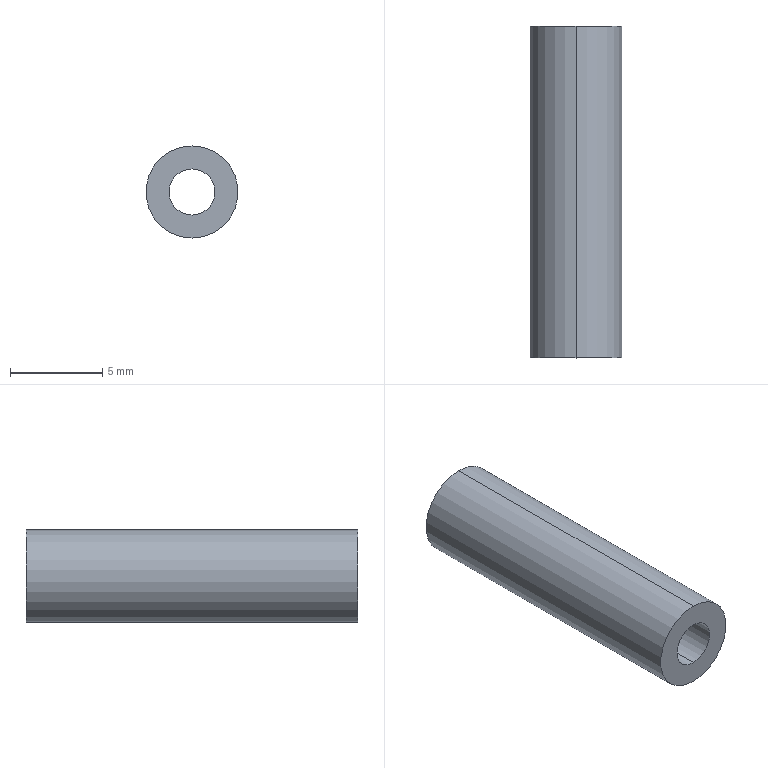Part | SolidWorks | features Extrusion 1, HoleWzd 1 | 1 solid | 6 faces | box 5 x 18 x 5 mm | volume 265.072 mm3 | cylinder 4 | plane 2 | commonest cylinder face diameters 2.5 x2 5 x2
STEP:
#1=CARTESIAN_POINT('',(0.,0.,-1.25));
#2=VERTEX_POINT('',#1);
#3=CARTESIAN_POINT('',(0.,0.,1.25));
#4=VERTEX_POINT('',#3);
#5=CARTESIAN_POINT('',(0.,0.,0.));
#6=DIRECTION('',(0.,1.,0.));
#7=DIRECTION('',(0.,0.,1.));
#8=AXIS2_PLACEMENT_3D('',#5,#6,#7);
#9=CIRCLE('',#8,1.25);
#10=EDGE_CURVE('',#2,#4,#9,.T.);
#11=ORIENTED_EDGE('',*,*,#10,.F.);
#12=CARTESIAN_POINT('',(0.,18.,-1.25));
#13=VERTEX_POINT('',#12);
#14=CARTESIAN_POINT('',(0.,18.,-1.25));
#15=DIRECTION('',(0.,1.,0.));
#16=VECTOR('',#15,1000.);
#17=LINE('',#14,#16);
#18=EDGE_CURVE('',#2,#13,#17,.T.);
#19=ORIENTED_EDGE('',*,*,#18,.T.);
#20=CARTESIAN_POINT('',(0.,18.,1.25));
#21=VERTEX_POINT('',#20);
#22=CARTESIAN_POINT('',(0.,18.,0.));
#23=DIRECTION('',(0.,1.,0.));
#24=DIRECTION('',(0.,0.,1.));
#25=AXIS2_PLACEMENT_3D('',#22,#23,#24);
#26=CIRCLE('',#25,1.25);
#27=EDGE_CURVE('',#13,#21,#26,.T.);
#28=ORIENTED_EDGE('',*,*,#27,.T.);
#29=CARTESIAN_POINT('',(0.,18.,1.25));
#30=DIRECTION('',(0.,1.,0.));
#31=VECTOR('',#30,1000.);
#32=LINE('',#29,#31);
#33=EDGE_CURVE('',#4,#21,#32,.T.);
#34=ORIENTED_EDGE('',*,*,#33,.F.);
#35=EDGE_LOOP('',(#11,#19,#28,#34));
#36=FACE_OUTER_BOUND('',#35,.T.);
#37=CARTESIAN_POINT('',(0.,18.,0.));
#38=DIRECTION('',(0.,1.,0.));
#39=DIRECTION('',(0.,0.,1.));
#40=AXIS2_PLACEMENT_3D('',#37,#38,#39);
#41=CYLINDRICAL_SURFACE('',#40,1.25);
#42=ADVANCED_FACE('',(#36),#41,.F.);
#43=CARTESIAN_POINT('',(0.,18.,2.5));
#44=VERTEX_POINT('',#43);
#45=CARTESIAN_POINT('',(0.,18.,-2.5));
#46=VERTEX_POINT('',#45);
#47=CARTESIAN_POINT('',(0.,18.,0.));
#48=DIRECTION('',(0.,1.,0.));
#49=DIRECTION('',(0.,0.,1.));
#50=AXIS2_PLACEMENT_3D('',#47,#48,#49);
#51=CIRCLE('',#50,2.5);
#52=EDGE_CURVE('',#44,#46,#51,.T.);
#53=ORIENTED_EDGE('',*,*,#52,.F.);
#54=CARTESIAN_POINT('',(0.,0.,2.5));
#55=VERTEX_POINT('',#54);
#56=CARTESIAN_POINT('',(0.,18.,2.5));
#57=DIRECTION('',(0.,-1.,0.));
#58=VECTOR('',#57,1000.);
#59=LINE('',#56,#58);
#60=EDGE_CURVE('',#44,#55,#59,.T.);
#61=ORIENTED_EDGE('',*,*,#60,.T.);
#62=CARTESIAN_POINT('',(0.,0.,-2.5));
#63=VERTEX_POINT('',#62);
#64=CARTESIAN_POINT('',(0.,0.,0.));
#65=DIRECTION('',(0.,1.,0.));
#66=DIRECTION('',(0.,0.,1.));
#67=AXIS2_PLACEMENT_3D('',#64,#65,#66);
#68=CIRCLE('',#67,2.5);
#69=EDGE_CURVE('',#55,#63,#68,.T.);
#70=ORIENTED_EDGE('',*,*,#69,.T.);
#71=CARTESIAN_POINT('',(0.,18.,-2.5));
#72=DIRECTION('',(0.,-1.,0.));
#73=VECTOR('',#72,1000.);
#74=LINE('',#71,#73);
#75=EDGE_CURVE('',#46,#63,#74,.T.);
#76=ORIENTED_EDGE('',*,*,#75,.F.);
#77=EDGE_LOOP('',(#53,#61,#70,#76));
#78=FACE_OUTER_BOUND('',#77,.T.);
#79=CARTESIAN_POINT('',(0.,18.,0.));
#80=DIRECTION('',(0.,-1.,0.));
#81=DIRECTION('',(0.,0.,-1.));
#82=AXIS2_PLACEMENT_3D('',#79,#80,#81);
#83=CYLINDRICAL_SURFACE('',#82,2.5);
#84=ADVANCED_FACE('',(#78),#83,.T.);
#85=ORIENTED_EDGE('',*,*,#60,.F.);
#86=CARTESIAN_POINT('',(0.,18.,0.));
#87=DIRECTION('',(0.,1.,0.));
#88=DIRECTION('',(0.,0.,1.));
#89=AXIS2_PLACEMENT_3D('',#86,#87,#88);
#90=CIRCLE('',#89,2.5);
#91=EDGE_CURVE('',#46,#44,#90,.T.);
#92=ORIENTED_EDGE('',*,*,#91,.F.);
#93=ORIENTED_EDGE('',*,*,#75,.T.);
#94=CARTESIAN_POINT('',(0.,0.,0.));
#95=DIRECTION('',(0.,1.,0.));
#96=DIRECTION('',(0.,0.,1.));
#97=AXIS2_PLACEMENT_3D('',#94,#95,#96);
#98=CIRCLE('',#97,2.5);
#99=EDGE_CURVE('',#63,#55,#98,.T.);
#100=ORIENTED_EDGE('',*,*,#99,.T.);
#101=EDGE_LOOP('',(#85,#92,#93,#100));
#102=FACE_OUTER_BOUND('',#101,.T.);
#103=CARTESIAN_POINT('',(0.,18.,0.));
#104=DIRECTION('',(0.,-1.,0.));
#105=DIRECTION('',(0.,0.,-1.));
#106=AXIS2_PLACEMENT_3D('',#103,#104,#105);
#107=CYLINDRICAL_SURFACE('',#106,2.5);
#108=ADVANCED_FACE('',(#102),#107,.T.);
#109=CARTESIAN_POINT('',(0.,18.,0.));
#110=DIRECTION('',(0.,1.,0.));
#111=DIRECTION('',(0.,0.,1.));
#112=AXIS2_PLACEMENT_3D('',#109,#110,#111);
#113=CIRCLE('',#112,1.25);
#114=EDGE_CURVE('',#21,#13,#113,.T.);
#115=ORIENTED_EDGE('',*,*,#114,.F.);
#116=ORIENTED_EDGE('',*,*,#27,.F.);
#117=EDGE_LOOP('',(#115,#116));
#118=FACE_BOUND('',#117,.T.);
#119=ORIENTED_EDGE('',*,*,#91,.T.);
#120=ORIENTED_EDGE('',*,*,#52,.T.);
#121=EDGE_LOOP('',(#119,#120));
#122=FACE_OUTER_BOUND('',#121,.T.);
#123=CARTESIAN_POINT('',(0.,18.,0.));
#124=DIRECTION('',(0.,1.,0.));
#125=DIRECTION('',(0.,0.,1.));
#126=AXIS2_PLACEMENT_3D('',#123,#124,#125);
#127=PLANE('',#126);
#128=ADVANCED_FACE('',(#118,#122),#127,.T.);
#129=CARTESIAN_POINT('',(0.,0.,0.));
#130=DIRECTION('',(0.,1.,0.));
#131=DIRECTION('',(0.,0.,1.));
#132=AXIS2_PLACEMENT_3D('',#129,#130,#131);
#133=CIRCLE('',#132,1.25);
#134=EDGE_CURVE('',#4,#2,#133,.T.);
#135=ORIENTED_EDGE('',*,*,#134,.T.);
#136=ORIENTED_EDGE('',*,*,#10,.T.);
#137=EDGE_LOOP('',(#135,#136));
#138=FACE_BOUND('',#137,.T.);
#139=ORIENTED_EDGE('',*,*,#99,.F.);
#140=ORIENTED_EDGE('',*,*,#69,.F.);
#141=EDGE_LOOP('',(#139,#140));
#142=FACE_OUTER_BOUND('',#141,.T.);
#143=CARTESIAN_POINT('',(0.,0.,0.));
#144=DIRECTION('',(0.,1.,0.));
#145=DIRECTION('',(0.,0.,1.));
#146=AXIS2_PLACEMENT_3D('',#143,#144,#145);
#147=PLANE('',#146);
#148=ADVANCED_FACE('',(#138,#142),#147,.F.);
#149=ORIENTED_EDGE('',*,*,#18,.F.);
#150=ORIENTED_EDGE('',*,*,#134,.F.);
#151=ORIENTED_EDGE('',*,*,#33,.T.);
#152=ORIENTED_EDGE('',*,*,#114,.T.);
#153=EDGE_LOOP('',(#149,#150,#151,#152));
#154=FACE_OUTER_BOUND('',#153,.T.);
#155=CARTESIAN_POINT('',(0.,18.,0.));
#156=DIRECTION('',(0.,1.,0.));
#157=DIRECTION('',(0.,0.,1.));
#158=AXIS2_PLACEMENT_3D('',#155,#156,#157);
#159=CYLINDRICAL_SURFACE('',#158,1.25);
#160=ADVANCED_FACE('',(#154),#159,.F.);
#161=CLOSED_SHELL('',(#42,#84,#108,#128,#148,#160));
#162=MANIFOLD_SOLID_BREP('',#161);
#163=CARTESIAN_POINT('',(0.,0.,0.));
#164=DIRECTION('',(0.,0.,1.));
#165=DIRECTION('',(1.,0.,0.));
#166=AXIS2_PLACEMENT_3D('',#163,#164,#165);
#167=(LENGTH_UNIT()NAMED_UNIT(*)SI_UNIT(.MILLI.,.METRE.));
#168=UNCERTAINTY_MEASURE_WITH_UNIT(LENGTH_MEASURE(0.00001),#167,'','');
#169=(NAMED_UNIT(*)PLANE_ANGLE_UNIT()SI_UNIT($,.RADIAN.));
#170=(NAMED_UNIT(*)SI_UNIT($,.STERADIAN.)SOLID_ANGLE_UNIT());
#171=(GEOMETRIC_REPRESENTATION_CONTEXT(3)GLOBAL_UNCERTAINTY_ASSIGNED_CONTEXT((#168))GLOBAL_UNIT_ASSIGNED_CONTEXT((#167,#169,#170))REPRESENTATION_CONTEXT('',''));
#172=ADVANCED_BREP_SHAPE_REPRESENTATION('',(#162,#166),#171);